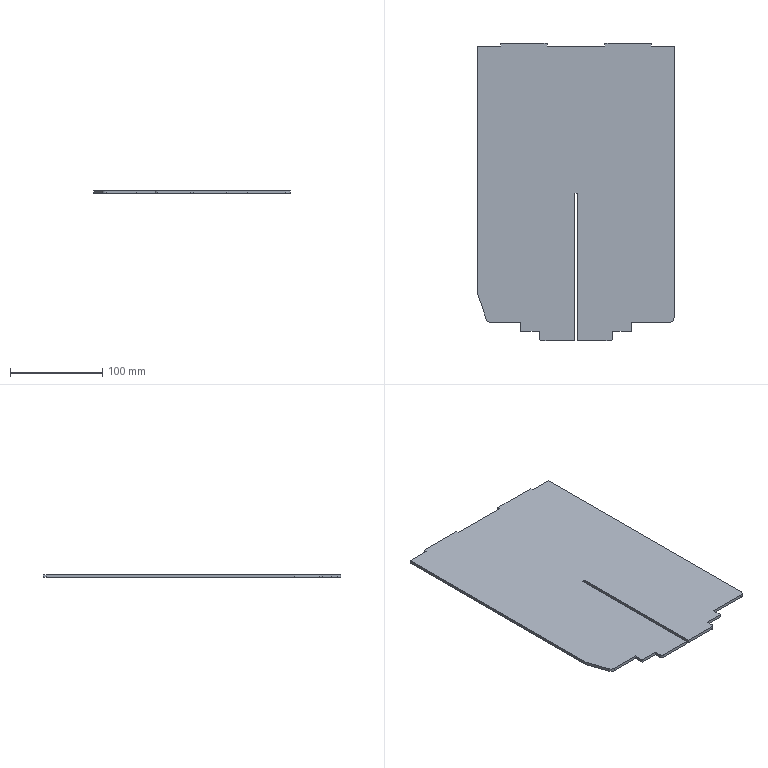Part | SolidWorks | features FlatPattern 1, SMBaseFlange 1, SheetMetal 1 | 1 solid | 31 faces | box 213 x 323 x 3.2 mm | volume 209682 mm3 | plane 27 | cylinder 4 | commonest cylinder face diameters 6 x2 10 x2
STEP:
#1=CARTESIAN_POINT('',(-107.314,104.189,0.));
#2=VERTEX_POINT('',#1);
#3=CARTESIAN_POINT('',(-132.314,104.189,0.));
#4=VERTEX_POINT('',#3);
#5=CARTESIAN_POINT('',(-107.314,104.189,0.));
#6=DIRECTION('',(-1.,0.,0.));
#7=VECTOR('',#6,1000.);
#8=LINE('',#5,#7);
#9=EDGE_CURVE('',#2,#4,#8,.T.);
#10=ORIENTED_EDGE('',*,*,#9,.T.);
#11=CARTESIAN_POINT('',(-132.314,104.189,3.2));
#12=VERTEX_POINT('',#11);
#13=CARTESIAN_POINT('',(-132.314,104.189,3.2));
#14=DIRECTION('',(0.,0.,-1.));
#15=VECTOR('',#14,1000.);
#16=LINE('',#13,#15);
#17=EDGE_CURVE('',#12,#4,#16,.T.);
#18=ORIENTED_EDGE('',*,*,#17,.F.);
#19=CARTESIAN_POINT('',(-107.314,104.189,3.2));
#20=VERTEX_POINT('',#19);
#21=CARTESIAN_POINT('',(-107.314,104.189,3.2));
#22=DIRECTION('',(-1.,0.,0.));
#23=VECTOR('',#22,1000.);
#24=LINE('',#21,#23);
#25=EDGE_CURVE('',#20,#12,#24,.T.);
#26=ORIENTED_EDGE('',*,*,#25,.F.);
#27=CARTESIAN_POINT('',(-107.314,104.189,3.2));
#28=DIRECTION('',(0.,0.,-1.));
#29=VECTOR('',#28,1000.);
#30=LINE('',#27,#29);
#31=EDGE_CURVE('',#20,#2,#30,.T.);
#32=ORIENTED_EDGE('',*,*,#31,.T.);
#33=EDGE_LOOP('',(#10,#18,#26,#32));
#34=FACE_OUTER_BOUND('',#33,.T.);
#35=CARTESIAN_POINT('',(-107.314,104.189,3.2));
#36=DIRECTION('',(0.,-1.,0.));
#37=DIRECTION('',(0.,0.,-1.));
#38=AXIS2_PLACEMENT_3D('',#35,#36,#37);
#39=PLANE('',#38);
#40=ADVANCED_FACE('',(#34),#39,.F.);
#41=CARTESIAN_POINT('',(-132.314,-165.811,0.));
#42=VERTEX_POINT('',#41);
#43=CARTESIAN_POINT('',(-132.314,-165.811,0.));
#44=DIRECTION('',(0.,-1.,0.));
#45=VECTOR('',#44,1000.);
#46=LINE('',#43,#45);
#47=EDGE_CURVE('',#4,#42,#46,.T.);
#48=ORIENTED_EDGE('',*,*,#47,.T.);
#49=CARTESIAN_POINT('',(-132.314,-165.811,3.2));
#50=VERTEX_POINT('',#49);
#51=CARTESIAN_POINT('',(-132.314,-165.811,3.2));
#52=DIRECTION('',(0.,0.,-1.));
#53=VECTOR('',#52,1000.);
#54=LINE('',#51,#53);
#55=EDGE_CURVE('',#50,#42,#54,.T.);
#56=ORIENTED_EDGE('',*,*,#55,.F.);
#57=CARTESIAN_POINT('',(-132.314,-165.811,3.2));
#58=DIRECTION('',(0.,-1.,0.));
#59=VECTOR('',#58,1000.);
#60=LINE('',#57,#59);
#61=EDGE_CURVE('',#12,#50,#60,.T.);
#62=ORIENTED_EDGE('',*,*,#61,.F.);
#63=ORIENTED_EDGE('',*,*,#17,.T.);
#64=EDGE_LOOP('',(#48,#56,#62,#63));
#65=FACE_OUTER_BOUND('',#64,.T.);
#66=CARTESIAN_POINT('',(-132.314,-165.811,3.2));
#67=DIRECTION('',(1.,0.,0.));
#68=DIRECTION('',(0.,0.,-1.));
#69=AXIS2_PLACEMENT_3D('',#66,#67,#68);
#70=PLANE('',#69);
#71=ADVANCED_FACE('',(#65),#70,.F.);
#72=CARTESIAN_POINT('',(-123.453,-192.392,0.));
#73=VERTEX_POINT('',#72);
#74=CARTESIAN_POINT('',(-123.453,-192.392,0.));
#75=DIRECTION('',(0.3162,-0.9487,0.));
#76=VECTOR('',#75,1000.);
#77=LINE('',#74,#76);
#78=EDGE_CURVE('',#42,#73,#77,.T.);
#79=ORIENTED_EDGE('',*,*,#78,.T.);
#80=CARTESIAN_POINT('',(-123.453,-192.392,3.2));
#81=VERTEX_POINT('',#80);
#82=CARTESIAN_POINT('',(-123.453,-192.392,3.2));
#83=DIRECTION('',(0.,0.,-1.));
#84=VECTOR('',#83,1000.);
#85=LINE('',#82,#84);
#86=EDGE_CURVE('',#81,#73,#85,.T.);
#87=ORIENTED_EDGE('',*,*,#86,.F.);
#88=CARTESIAN_POINT('',(-123.453,-192.392,3.2));
#89=DIRECTION('',(0.3162,-0.9487,0.));
#90=VECTOR('',#89,1000.);
#91=LINE('',#88,#90);
#92=EDGE_CURVE('',#50,#81,#91,.T.);
#93=ORIENTED_EDGE('',*,*,#92,.F.);
#94=ORIENTED_EDGE('',*,*,#55,.T.);
#95=EDGE_LOOP('',(#79,#87,#93,#94));
#96=FACE_OUTER_BOUND('',#95,.T.);
#97=CARTESIAN_POINT('',(-123.453,-192.392,3.2));
#98=DIRECTION('',(0.9487,0.3162,0.));
#99=DIRECTION('',(-0.3162,0.9487,0.));
#100=AXIS2_PLACEMENT_3D('',#97,#98,#99);
#101=PLANE('',#100);
#102=ADVANCED_FACE('',(#96),#101,.F.);
#103=CARTESIAN_POINT('',(-118.71,-195.811,0.));
#104=VERTEX_POINT('',#103);
#105=CARTESIAN_POINT('',(-118.71,-190.811,0.));
#106=DIRECTION('',(0.,0.,1.));
#107=DIRECTION('',(1.,0.,0.));
#108=AXIS2_PLACEMENT_3D('',#105,#106,#107);
#109=CIRCLE('',#108,5.);
#110=EDGE_CURVE('',#73,#104,#109,.T.);
#111=ORIENTED_EDGE('',*,*,#110,.T.);
#112=CARTESIAN_POINT('',(-118.71,-195.811,3.2));
#113=VERTEX_POINT('',#112);
#114=CARTESIAN_POINT('',(-118.71,-195.811,3.2));
#115=DIRECTION('',(0.,0.,-1.));
#116=VECTOR('',#115,1000.);
#117=LINE('',#114,#116);
#118=EDGE_CURVE('',#113,#104,#117,.T.);
#119=ORIENTED_EDGE('',*,*,#118,.F.);
#120=CARTESIAN_POINT('',(-118.71,-190.811,3.2));
#121=DIRECTION('',(0.,0.,1.));
#122=DIRECTION('',(1.,0.,0.));
#123=AXIS2_PLACEMENT_3D('',#120,#121,#122);
#124=CIRCLE('',#123,5.);
#125=EDGE_CURVE('',#81,#113,#124,.T.);
#126=ORIENTED_EDGE('',*,*,#125,.F.);
#127=ORIENTED_EDGE('',*,*,#86,.T.);
#128=EDGE_LOOP('',(#111,#119,#126,#127));
#129=FACE_OUTER_BOUND('',#128,.T.);
#130=CARTESIAN_POINT('',(-118.71,-190.811,3.2));
#131=DIRECTION('',(0.,0.,-1.));
#132=DIRECTION('',(-1.,0.,0.));
#133=AXIS2_PLACEMENT_3D('',#130,#131,#132);
#134=CYLINDRICAL_SURFACE('',#133,5.);
#135=ADVANCED_FACE('',(#129),#134,.T.);
#136=CARTESIAN_POINT('',(-85.814,-195.811,0.));
#137=VERTEX_POINT('',#136);
#138=CARTESIAN_POINT('',(-85.814,-195.811,0.));
#139=DIRECTION('',(1.,0.,0.));
#140=VECTOR('',#139,1000.);
#141=LINE('',#138,#140);
#142=EDGE_CURVE('',#104,#137,#141,.T.);
#143=ORIENTED_EDGE('',*,*,#142,.T.);
#144=CARTESIAN_POINT('',(-85.814,-195.811,3.2));
#145=VERTEX_POINT('',#144);
#146=CARTESIAN_POINT('',(-85.814,-195.811,3.2));
#147=DIRECTION('',(0.,0.,-1.));
#148=VECTOR('',#147,1000.);
#149=LINE('',#146,#148);
#150=EDGE_CURVE('',#145,#137,#149,.T.);
#151=ORIENTED_EDGE('',*,*,#150,.F.);
#152=CARTESIAN_POINT('',(-85.814,-195.811,3.2));
#153=DIRECTION('',(1.,0.,0.));
#154=VECTOR('',#153,1000.);
#155=LINE('',#152,#154);
#156=EDGE_CURVE('',#113,#145,#155,.T.);
#157=ORIENTED_EDGE('',*,*,#156,.F.);
#158=ORIENTED_EDGE('',*,*,#118,.T.);
#159=EDGE_LOOP('',(#143,#151,#157,#158));
#160=FACE_OUTER_BOUND('',#159,.T.);
#161=CARTESIAN_POINT('',(-85.814,-195.811,3.2));
#162=DIRECTION('',(0.,1.,0.));
#163=DIRECTION('',(-1.,0.,0.));
#164=AXIS2_PLACEMENT_3D('',#161,#162,#163);
#165=PLANE('',#164);
#166=ADVANCED_FACE('',(#160),#165,.F.);
#167=CARTESIAN_POINT('',(-85.814,-205.811,0.));
#168=VERTEX_POINT('',#167);
#169=CARTESIAN_POINT('',(-85.814,-205.811,0.));
#170=DIRECTION('',(0.,-1.,0.));
#171=VECTOR('',#170,1000.);
#172=LINE('',#169,#171);
#173=EDGE_CURVE('',#137,#168,#172,.T.);
#174=ORIENTED_EDGE('',*,*,#173,.T.);
#175=CARTESIAN_POINT('',(-85.814,-205.811,3.2));
#176=VERTEX_POINT('',#175);
#177=CARTESIAN_POINT('',(-85.814,-205.811,3.2));
#178=DIRECTION('',(0.,0.,-1.));
#179=VECTOR('',#178,1000.);
#180=LINE('',#177,#179);
#181=EDGE_CURVE('',#176,#168,#180,.T.);
#182=ORIENTED_EDGE('',*,*,#181,.F.);
#183=CARTESIAN_POINT('',(-85.814,-205.811,3.2));
#184=DIRECTION('',(0.,-1.,0.));
#185=VECTOR('',#184,1000.);
#186=LINE('',#183,#185);
#187=EDGE_CURVE('',#145,#176,#186,.T.);
#188=ORIENTED_EDGE('',*,*,#187,.F.);
#189=ORIENTED_EDGE('',*,*,#150,.T.);
#190=EDGE_LOOP('',(#174,#182,#188,#189));
#191=FACE_OUTER_BOUND('',#190,.T.);
#192=CARTESIAN_POINT('',(-85.814,-205.811,3.2));
#193=DIRECTION('',(1.,0.,0.));
#194=DIRECTION('',(0.,1.,0.));
#195=AXIS2_PLACEMENT_3D('',#192,#193,#194);
#196=PLANE('',#195);
#197=ADVANCED_FACE('',(#191),#196,.F.);
#198=CARTESIAN_POINT('',(-65.814,-205.811,0.));
#199=VERTEX_POINT('',#198);
#200=CARTESIAN_POINT('',(-65.814,-205.811,0.));
#201=DIRECTION('',(1.,0.,0.));
#202=VECTOR('',#201,1000.);
#203=LINE('',#200,#202);
#204=EDGE_CURVE('',#168,#199,#203,.T.);
#205=ORIENTED_EDGE('',*,*,#204,.T.);
#206=CARTESIAN_POINT('',(-65.814,-205.811,3.2));
#207=VERTEX_POINT('',#206);
#208=CARTESIAN_POINT('',(-65.814,-205.811,3.2));
#209=DIRECTION('',(0.,0.,-1.));
#210=VECTOR('',#209,1000.);
#211=LINE('',#208,#210);
#212=EDGE_CURVE('',#207,#199,#211,.T.);
#213=ORIENTED_EDGE('',*,*,#212,.F.);
#214=CARTESIAN_POINT('',(-65.814,-205.811,3.2));
#215=DIRECTION('',(1.,0.,0.));
#216=VECTOR('',#215,1000.);
#217=LINE('',#214,#216);
#218=EDGE_CURVE('',#176,#207,#217,.T.);
#219=ORIENTED_EDGE('',*,*,#218,.F.);
#220=ORIENTED_EDGE('',*,*,#181,.T.);
#221=EDGE_LOOP('',(#205,#213,#219,#220));
#222=FACE_OUTER_BOUND('',#221,.T.);
#223=CARTESIAN_POINT('',(-65.814,-205.811,3.2));
#224=DIRECTION('',(0.,1.,0.));
#225=DIRECTION('',(-1.,0.,0.));
#226=AXIS2_PLACEMENT_3D('',#223,#224,#225);
#227=PLANE('',#226);
#228=ADVANCED_FACE('',(#222),#227,.F.);
#229=CARTESIAN_POINT('',(-65.814,-212.811,0.));
#230=VERTEX_POINT('',#229);
#231=CARTESIAN_POINT('',(-65.814,-212.811,0.));
#232=DIRECTION('',(0.,-1.,0.));
#233=VECTOR('',#232,1000.);
#234=LINE('',#231,#233);
#235=EDGE_CURVE('',#199,#230,#234,.T.);
#236=ORIENTED_EDGE('',*,*,#235,.T.);
#237=CARTESIAN_POINT('',(-65.814,-212.811,3.2));
#238=VERTEX_POINT('',#237);
#239=CARTESIAN_POINT('',(-65.814,-212.811,3.2));
#240=DIRECTION('',(0.,0.,-1.));
#241=VECTOR('',#240,1000.);
#242=LINE('',#239,#241);
#243=EDGE_CURVE('',#238,#230,#242,.T.);
#244=ORIENTED_EDGE('',*,*,#243,.F.);
#245=CARTESIAN_POINT('',(-65.814,-212.811,3.2));
#246=DIRECTION('',(0.,-1.,0.));
#247=VECTOR('',#246,1000.);
#248=LINE('',#245,#247);
#249=EDGE_CURVE('',#207,#238,#248,.T.);
#250=ORIENTED_EDGE('',*,*,#249,.F.);
#251=ORIENTED_EDGE('',*,*,#212,.T.);
#252=EDGE_LOOP('',(#236,#244,#250,#251));
#253=FACE_OUTER_BOUND('',#252,.T.);
#254=CARTESIAN_POINT('',(-65.814,-212.811,3.2));
#255=DIRECTION('',(1.,0.,0.));
#256=DIRECTION('',(0.,0.,-1.));
#257=AXIS2_PLACEMENT_3D('',#254,#255,#256);
#258=PLANE('',#257);
#259=ADVANCED_FACE('',(#253),#258,.F.);
#260=CARTESIAN_POINT('',(-62.814,-215.811,0.));
#261=VERTEX_POINT('',#260);
#262=CARTESIAN_POINT('',(-62.814,-212.811,0.));
#263=DIRECTION('',(0.,0.,1.));
#264=DIRECTION('',(-1.,0.,0.));
#265=AXIS2_PLACEMENT_3D('',#262,#263,#264);
#266=CIRCLE('',#265,3.);
#267=EDGE_CURVE('',#230,#261,#266,.T.);
#268=ORIENTED_EDGE('',*,*,#267,.T.);
#269=CARTESIAN_POINT('',(-62.814,-215.811,3.2));
#270=VERTEX_POINT('',#269);
#271=CARTESIAN_POINT('',(-62.814,-215.811,3.2));
#272=DIRECTION('',(0.,0.,-1.));
#273=VECTOR('',#272,1000.);
#274=LINE('',#271,#273);
#275=EDGE_CURVE('',#270,#261,#274,.T.);
#276=ORIENTED_EDGE('',*,*,#275,.F.);
#277=CARTESIAN_POINT('',(-62.814,-212.811,3.2));
#278=DIRECTION('',(0.,0.,1.));
#279=DIRECTION('',(-1.,0.,0.));
#280=AXIS2_PLACEMENT_3D('',#277,#278,#279);
#281=CIRCLE('',#280,3.);
#282=EDGE_CURVE('',#238,#270,#281,.T.);
#283=ORIENTED_EDGE('',*,*,#282,.F.);
#284=ORIENTED_EDGE('',*,*,#243,.T.);
#285=EDGE_LOOP('',(#268,#276,#283,#284));
#286=FACE_OUTER_BOUND('',#285,.T.);
#287=CARTESIAN_POINT('',(-62.814,-212.811,3.2));
#288=DIRECTION('',(0.,0.,-1.));
#289=DIRECTION('',(-1.,0.,0.));
#290=AXIS2_PLACEMENT_3D('',#287,#288,#289);
#291=CYLINDRICAL_SURFACE('',#290,3.);
#292=ADVANCED_FACE('',(#286),#291,.T.);
#293=CARTESIAN_POINT('',(-27.414,-215.811,0.));
#294=VERTEX_POINT('',#293);
#295=CARTESIAN_POINT('',(-27.414,-215.811,0.));
#296=DIRECTION('',(1.,0.,0.));
#297=VECTOR('',#296,1000.);
#298=LINE('',#295,#297);
#299=EDGE_CURVE('',#261,#294,#298,.T.);
#300=ORIENTED_EDGE('',*,*,#299,.T.);
#301=CARTESIAN_POINT('',(-27.414,-215.811,3.2));
#302=VERTEX_POINT('',#301);
#303=CARTESIAN_POINT('',(-27.414,-215.811,3.2));
#304=DIRECTION('',(0.,0.,-1.));
#305=VECTOR('',#304,1000.);
#306=LINE('',#303,#305);
#307=EDGE_CURVE('',#302,#294,#306,.T.);
#308=ORIENTED_EDGE('',*,*,#307,.F.);
#309=CARTESIAN_POINT('',(-27.414,-215.811,3.2));
#310=DIRECTION('',(1.,0.,0.));
#311=VECTOR('',#310,1000.);
#312=LINE('',#309,#311);
#313=EDGE_CURVE('',#270,#302,#312,.T.);
#314=ORIENTED_EDGE('',*,*,#313,.F.);
#315=ORIENTED_EDGE('',*,*,#275,.T.);
#316=EDGE_LOOP('',(#300,#308,#314,#315));
#317=FACE_OUTER_BOUND('',#316,.T.);
#318=CARTESIAN_POINT('',(-27.414,-215.811,3.2));
#319=DIRECTION('',(0.,1.,0.));
#320=DIRECTION('',(0.,0.,1.));
#321=AXIS2_PLACEMENT_3D('',#318,#319,#320);
#322=PLANE('',#321);
#323=ADVANCED_FACE('',(#317),#322,.F.);
#324=CARTESIAN_POINT('',(-27.414,-55.611,0.));
#325=VERTEX_POINT('',#324);
#326=CARTESIAN_POINT('',(-27.414,-55.611,0.));
#327=DIRECTION('',(0.,1.,0.));
#328=VECTOR('',#327,1000.);
#329=LINE('',#326,#328);
#330=EDGE_CURVE('',#294,#325,#329,.T.);
#331=ORIENTED_EDGE('',*,*,#330,.T.);
#332=CARTESIAN_POINT('',(-27.414,-55.611,3.2));
#333=VERTEX_POINT('',#332);
#334=CARTESIAN_POINT('',(-27.414,-55.611,3.2));
#335=DIRECTION('',(0.,0.,-1.));
#336=VECTOR('',#335,1000.);
#337=LINE('',#334,#336);
#338=EDGE_CURVE('',#333,#325,#337,.T.);
#339=ORIENTED_EDGE('',*,*,#338,.F.);
#340=CARTESIAN_POINT('',(-27.414,-55.611,3.2));
#341=DIRECTION('',(0.,1.,0.));
#342=VECTOR('',#341,1000.);
#343=LINE('',#340,#342);
#344=EDGE_CURVE('',#302,#333,#343,.T.);
#345=ORIENTED_EDGE('',*,*,#344,.F.);
#346=ORIENTED_EDGE('',*,*,#307,.T.);
#347=EDGE_LOOP('',(#331,#339,#345,#346));
#348=FACE_OUTER_BOUND('',#347,.T.);
#349=CARTESIAN_POINT('',(-27.414,-55.611,3.2));
#350=DIRECTION('',(-1.,0.,0.));
#351=DIRECTION('',(0.,0.,1.));
#352=AXIS2_PLACEMENT_3D('',#349,#350,#351);
#353=PLANE('',#352);
#354=ADVANCED_FACE('',(#348),#353,.F.);
#355=CARTESIAN_POINT('',(-24.214,-55.611,0.));
#356=VERTEX_POINT('',#355);
#357=CARTESIAN_POINT('',(-24.214,-55.611,0.));
#358=DIRECTION('',(1.,0.,0.));
#359=VECTOR('',#358,1000.);
#360=LINE('',#357,#359);
#361=EDGE_CURVE('',#325,#356,#360,.T.);
#362=ORIENTED_EDGE('',*,*,#361,.T.);
#363=CARTESIAN_POINT('',(-24.214,-55.611,3.2));
#364=VERTEX_POINT('',#363);
#365=CARTESIAN_POINT('',(-24.214,-55.611,3.2));
#366=DIRECTION('',(0.,0.,-1.));
#367=VECTOR('',#366,1000.);
#368=LINE('',#365,#367);
#369=EDGE_CURVE('',#364,#356,#368,.T.);
#370=ORIENTED_EDGE('',*,*,#369,.F.);
#371=CARTESIAN_POINT('',(-24.214,-55.611,3.2));
#372=DIRECTION('',(1.,0.,0.));
#373=VECTOR('',#372,1000.);
#374=LINE('',#371,#373);
#375=EDGE_CURVE('',#333,#364,#374,.T.);
#376=ORIENTED_EDGE('',*,*,#375,.F.);
#377=ORIENTED_EDGE('',*,*,#338,.T.);
#378=EDGE_LOOP('',(#362,#370,#376,#377));
#379=FACE_OUTER_BOUND('',#378,.T.);
#380=CARTESIAN_POINT('',(-24.214,-55.611,3.2));
#381=DIRECTION('',(0.,1.,0.));
#382=DIRECTION('',(-1.,0.,0.));
#383=AXIS2_PLACEMENT_3D('',#380,#381,#382);
#384=PLANE('',#383);
#385=ADVANCED_FACE('',(#379),#384,.F.);
#386=CARTESIAN_POINT('',(-24.214,-215.811,0.));
#387=VERTEX_POINT('',#386);
#388=CARTESIAN_POINT('',(-24.214,-215.811,0.));
#389=DIRECTION('',(0.,-1.,0.));
#390=VECTOR('',#389,1000.);
#391=LINE('',#388,#390);
#392=EDGE_CURVE('',#356,#387,#391,.T.);
#393=ORIENTED_EDGE('',*,*,#392,.T.);
#394=CARTESIAN_POINT('',(-24.214,-215.811,3.2));
#395=VERTEX_POINT('',#394);
#396=CARTESIAN_POINT('',(-24.214,-215.811,3.2));
#397=DIRECTION('',(0.,0.,-1.));
#398=VECTOR('',#397,1000.);
#399=LINE('',#396,#398);
#400=EDGE_CURVE('',#395,#387,#399,.T.);
#401=ORIENTED_EDGE('',*,*,#400,.F.);
#402=CARTESIAN_POINT('',(-24.214,-215.811,3.2));
#403=DIRECTION('',(0.,-1.,0.));
#404=VECTOR('',#403,1000.);
#405=LINE('',#402,#404);
#406=EDGE_CURVE('',#364,#395,#405,.T.);
#407=ORIENTED_EDGE('',*,*,#406,.F.);
#408=ORIENTED_EDGE('',*,*,#369,.T.);
#409=EDGE_LOOP('',(#393,#401,#407,#408));
#410=FACE_OUTER_BOUND('',#409,.T.);
#411=CARTESIAN_POINT('',(-24.214,-215.811,3.2));
#412=DIRECTION('',(1.,0.,0.));
#413=DIRECTION('',(0.,1.,0.));
#414=AXIS2_PLACEMENT_3D('',#411,#412,#413);
#415=PLANE('',#414);
#416=ADVANCED_FACE('',(#410),#415,.F.);
#417=CARTESIAN_POINT('',(11.186,-215.811,0.));
#418=VERTEX_POINT('',#417);
#419=CARTESIAN_POINT('',(11.186,-215.811,0.));
#420=DIRECTION('',(1.,0.,0.));
#421=VECTOR('',#420,1000.);
#422=LINE('',#419,#421);
#423=EDGE_CURVE('',#387,#418,#422,.T.);
#424=ORIENTED_EDGE('',*,*,#423,.T.);
#425=CARTESIAN_POINT('',(11.186,-215.811,3.2));
#426=VERTEX_POINT('',#425);
#427=CARTESIAN_POINT('',(11.186,-215.811,3.2));
#428=DIRECTION('',(0.,0.,-1.));
#429=VECTOR('',#428,1000.);
#430=LINE('',#427,#429);
#431=EDGE_CURVE('',#426,#418,#430,.T.);
#432=ORIENTED_EDGE('',*,*,#431,.F.);
#433=CARTESIAN_POINT('',(11.186,-215.811,3.2));
#434=DIRECTION('',(1.,0.,0.));
#435=VECTOR('',#434,1000.);
#436=LINE('',#433,#435);
#437=EDGE_CURVE('',#395,#426,#436,.T.);
#438=ORIENTED_EDGE('',*,*,#437,.F.);
#439=ORIENTED_EDGE('',*,*,#400,.T.);
#440=EDGE_LOOP('',(#424,#432,#438,#439));
#441=FACE_OUTER_BOUND('',#440,.T.);
#442=CARTESIAN_POINT('',(11.186,-215.811,3.2));
#443=DIRECTION('',(0.,1.,0.));
#444=DIRECTION('',(-1.,0.,0.));
#445=AXIS2_PLACEMENT_3D('',#442,#443,#444);
#446=PLANE('',#445);
#447=ADVANCED_FACE('',(#441),#446,.F.);
#448=CARTESIAN_POINT('',(14.186,-212.811,0.));
#449=VERTEX_POINT('',#448);
#450=CARTESIAN_POINT('',(11.186,-212.811,0.));
#451=DIRECTION('',(0.,0.,1.));
#452=DIRECTION('',(-1.,0.,0.));
#453=AXIS2_PLACEMENT_3D('',#450,#451,#452);
#454=CIRCLE('',#453,3.);
#455=EDGE_CURVE('',#418,#449,#454,.T.);
#456=ORIENTED_EDGE('',*,*,#455,.T.);
#457=CARTESIAN_POINT('',(14.186,-212.811,3.2));
#458=VERTEX_POINT('',#457);
#459=CARTESIAN_POINT('',(14.186,-212.811,3.2));
#460=DIRECTION('',(0.,0.,-1.));
#461=VECTOR('',#460,1000.);
#462=LINE('',#459,#461);
#463=EDGE_CURVE('',#458,#449,#462,.T.);
#464=ORIENTED_EDGE('',*,*,#463,.F.);
#465=CARTESIAN_POINT('',(11.186,-212.811,3.2));
#466=DIRECTION('',(0.,0.,1.));
#467=DIRECTION('',(-1.,0.,0.));
#468=AXIS2_PLACEMENT_3D('',#465,#466,#467);
#469=CIRCLE('',#468,3.);
#470=EDGE_CURVE('',#426,#458,#469,.T.);
#471=ORIENTED_EDGE('',*,*,#470,.F.);
#472=ORIENTED_EDGE('',*,*,#431,.T.);
#473=EDGE_LOOP('',(#456,#464,#471,#472));
#474=FACE_OUTER_BOUND('',#473,.T.);
#475=CARTESIAN_POINT('',(11.186,-212.811,3.2));
#476=DIRECTION('',(0.,0.,-1.));
#477=DIRECTION('',(-1.,0.,0.));
#478=AXIS2_PLACEMENT_3D('',#475,#476,#477);
#479=CYLINDRICAL_SURFACE('',#478,3.);
#480=ADVANCED_FACE('',(#474),#479,.T.);
#481=CARTESIAN_POINT('',(14.186,-205.811,0.));
#482=VERTEX_POINT('',#481);
#483=CARTESIAN_POINT('',(14.186,-205.811,0.));
#484=DIRECTION('',(0.,1.,0.));
#485=VECTOR('',#484,1000.);
#486=LINE('',#483,#485);
#487=EDGE_CURVE('',#449,#482,#486,.T.);
#488=ORIENTED_EDGE('',*,*,#487,.T.);
#489=CARTESIAN_POINT('',(14.186,-205.811,3.2));
#490=VERTEX_POINT('',#489);
#491=CARTESIAN_POINT('',(14.186,-205.811,3.2));
#492=DIRECTION('',(0.,0.,-1.));
#493=VECTOR('',#492,1000.);
#494=LINE('',#491,#493);
#495=EDGE_CURVE('',#490,#482,#494,.T.);
#496=ORIENTED_EDGE('',*,*,#495,.F.);
#497=CARTESIAN_POINT('',(14.186,-205.811,3.2));
#498=DIRECTION('',(0.,1.,0.));
#499=VECTOR('',#498,1000.);
#500=LINE('',#497,#499);
#501=EDGE_CURVE('',#458,#490,#500,.T.);
#502=ORIENTED_EDGE('',*,*,#501,.F.);
#503=ORIENTED_EDGE('',*,*,#463,.T.);
#504=EDGE_LOOP('',(#488,#496,#502,#503));
#505=FACE_OUTER_BOUND('',#504,.T.);
#506=CARTESIAN_POINT('',(14.186,-205.811,3.2));
#507=DIRECTION('',(-1.,0.,0.));
#508=DIRECTION('',(0.,-1.,0.));
#509=AXIS2_PLACEMENT_3D('',#506,#507,#508);
#510=PLANE('',#509);
#511=ADVANCED_FACE('',(#505),#510,.F.);
#512=CARTESIAN_POINT('',(34.186,-205.811,0.));
#513=VERTEX_POINT('',#512);
#514=CARTESIAN_POINT('',(34.186,-205.811,0.));
#515=DIRECTION('',(1.,0.,0.));
#516=VECTOR('',#515,1000.);
#517=LINE('',#514,#516);
#518=EDGE_CURVE('',#482,#513,#517,.T.);
#519=ORIENTED_EDGE('',*,*,#518,.T.);
#520=CARTESIAN_POINT('',(34.186,-205.811,3.2));
#521=VERTEX_POINT('',#520);
#522=CARTESIAN_POINT('',(34.186,-205.811,3.2));
#523=DIRECTION('',(0.,0.,-1.));
#524=VECTOR('',#523,1000.);
#525=LINE('',#522,#524);
#526=EDGE_CURVE('',#521,#513,#525,.T.);
#527=ORIENTED_EDGE('',*,*,#526,.F.);
#528=CARTESIAN_POINT('',(34.186,-205.811,3.2));
#529=DIRECTION('',(1.,0.,0.));
#530=VECTOR('',#529,1000.);
#531=LINE('',#528,#530);
#532=EDGE_CURVE('',#490,#521,#531,.T.);
#533=ORIENTED_EDGE('',*,*,#532,.F.);
#534=ORIENTED_EDGE('',*,*,#495,.T.);
#535=EDGE_LOOP('',(#519,#527,#533,#534));
#536=FACE_OUTER_BOUND('',#535,.T.);
#537=CARTESIAN_POINT('',(34.186,-205.811,3.2));
#538=DIRECTION('',(0.,1.,0.));
#539=DIRECTION('',(-1.,0.,0.));
#540=AXIS2_PLACEMENT_3D('',#537,#538,#539);
#541=PLANE('',#540);
#542=ADVANCED_FACE('',(#536),#541,.F.);
#543=CARTESIAN_POINT('',(34.186,-195.811,0.));
#544=VERTEX_POINT('',#543);
#545=CARTESIAN_POINT('',(34.186,-195.811,0.));
#546=DIRECTION('',(0.,1.,0.));
#547=VECTOR('',#546,1000.);
#548=LINE('',#545,#547);
#549=EDGE_CURVE('',#513,#544,#548,.T.);
#550=ORIENTED_EDGE('',*,*,#549,.T.);
#551=CARTESIAN_POINT('',(34.186,-195.811,3.2));
#552=VERTEX_POINT('',#551);
#553=CARTESIAN_POINT('',(34.186,-195.811,3.2));
#554=DIRECTION('',(0.,0.,-1.));
#555=VECTOR('',#554,1000.);
#556=LINE('',#553,#555);
#557=EDGE_CURVE('',#552,#544,#556,.T.);
#558=ORIENTED_EDGE('',*,*,#557,.F.);
#559=CARTESIAN_POINT('',(34.186,-195.811,3.2));
#560=DIRECTION('',(0.,1.,0.));
#561=VECTOR('',#560,1000.);
#562=LINE('',#559,#561);
#563=EDGE_CURVE('',#521,#552,#562,.T.);
#564=ORIENTED_EDGE('',*,*,#563,.F.);
#565=ORIENTED_EDGE('',*,*,#526,.T.);
#566=EDGE_LOOP('',(#550,#558,#564,#565));
#567=FACE_OUTER_BOUND('',#566,.T.);
#568=CARTESIAN_POINT('',(34.186,-195.811,3.2));
#569=DIRECTION('',(-1.,0.,0.));
#570=DIRECTION('',(0.,-1.,0.));
#571=AXIS2_PLACEMENT_3D('',#568,#569,#570);
#572=PLANE('',#571);
#573=ADVANCED_FACE('',(#567),#572,.F.);
#574=CARTESIAN_POINT('',(75.686,-195.811,0.));
#575=VERTEX_POINT('',#574);
#576=CARTESIAN_POINT('',(75.686,-195.811,0.));
#577=DIRECTION('',(1.,0.,0.));
#578=VECTOR('',#577,1000.);
#579=LINE('',#576,#578);
#580=EDGE_CURVE('',#544,#575,#579,.T.);
#581=ORIENTED_EDGE('',*,*,#580,.T.);
#582=CARTESIAN_POINT('',(75.686,-195.811,3.2));
#583=VERTEX_POINT('',#582);
#584=CARTESIAN_POINT('',(75.686,-195.811,3.2));
#585=DIRECTION('',(0.,0.,-1.));
#586=VECTOR('',#585,1000.);
#587=LINE('',#584,#586);
#588=EDGE_CURVE('',#583,#575,#587,.T.);
#589=ORIENTED_EDGE('',*,*,#588,.F.);
#590=CARTESIAN_POINT('',(75.686,-195.811,3.2));
#591=DIRECTION('',(1.,0.,0.));
#592=VECTOR('',#591,1000.);
#593=LINE('',#590,#592);
#594=EDGE_CURVE('',#552,#583,#593,.T.);
#595=ORIENTED_EDGE('',*,*,#594,.F.);
#596=ORIENTED_EDGE('',*,*,#557,.T.);
#597=EDGE_LOOP('',(#581,#589,#595,#596));
#598=FACE_OUTER_BOUND('',#597,.T.);
#599=CARTESIAN_POINT('',(75.686,-195.811,3.2));
#600=DIRECTION('',(0.,1.,0.));
#601=DIRECTION('',(-1.,0.,0.));
#602=AXIS2_PLACEMENT_3D('',#599,#600,#601);
#603=PLANE('',#602);
#604=ADVANCED_FACE('',(#598),#603,.F.);
#605=CARTESIAN_POINT('',(80.686,-190.811,0.));
#606=VERTEX_POINT('',#605);
#607=CARTESIAN_POINT('',(75.686,-190.811,0.));
#608=DIRECTION('',(0.,0.,1.));
#609=DIRECTION('',(1.,0.,0.));
#610=AXIS2_PLACEMENT_3D('',#607,#608,#609);
#611=CIRCLE('',#610,5.);
#612=EDGE_CURVE('',#575,#606,#611,.T.);
#613=ORIENTED_EDGE('',*,*,#612,.T.);
#614=CARTESIAN_POINT('',(80.686,-190.811,3.2));
#615=VERTEX_POINT('',#614);
#616=CARTESIAN_POINT('',(80.686,-190.811,3.2));
#617=DIRECTION('',(0.,0.,-1.));
#618=VECTOR('',#617,1000.);
#619=LINE('',#616,#618);
#620=EDGE_CURVE('',#615,#606,#619,.T.);
#621=ORIENTED_EDGE('',*,*,#620,.F.);
#622=CARTESIAN_POINT('',(75.686,-190.811,3.2));
#623=DIRECTION('',(0.,0.,1.));
#624=DIRECTION('',(1.,0.,0.));
#625=AXIS2_PLACEMENT_3D('',#622,#623,#624);
#626=CIRCLE('',#625,5.);
#627=EDGE_CURVE('',#583,#615,#626,.T.);
#628=ORIENTED_EDGE('',*,*,#627,.F.);
#629=ORIENTED_EDGE('',*,*,#588,.T.);
#630=EDGE_LOOP('',(#613,#621,#628,#629));
#631=FACE_OUTER_BOUND('',#630,.T.);
#632=CARTESIAN_POINT('',(75.686,-190.811,3.2));
#633=DIRECTION('',(0.,0.,-1.));
#634=DIRECTION('',(-1.,0.,0.));
#635=AXIS2_PLACEMENT_3D('',#632,#633,#634);
#636=CYLINDRICAL_SURFACE('',#635,5.);
#637=ADVANCED_FACE('',(#631),#636,.T.);
#638=CARTESIAN_POINT('',(80.686,104.189,0.));
#639=VERTEX_POINT('',#638);
#640=CARTESIAN_POINT('',(80.686,-190.811,0.));
#641=DIRECTION('',(0.,1.,0.));
#642=VECTOR('',#641,1000.);
#643=LINE('',#640,#642);
#644=EDGE_CURVE('',#606,#639,#643,.T.);
#645=ORIENTED_EDGE('',*,*,#644,.T.);
#646=CARTESIAN_POINT('',(80.686,104.189,3.2));
#647=VERTEX_POINT('',#646);
#648=CARTESIAN_POINT('',(80.686,104.189,3.2));
#649=DIRECTION('',(0.,0.,-1.));
#650=VECTOR('',#649,1000.);
#651=LINE('',#648,#650);
#652=EDGE_CURVE('',#647,#639,#651,.T.);
#653=ORIENTED_EDGE('',*,*,#652,.F.);
#654=CARTESIAN_POINT('',(80.686,-190.811,3.2));
#655=DIRECTION('',(0.,1.,0.));
#656=VECTOR('',#655,1000.);
#657=LINE('',#654,#656);
#658=EDGE_CURVE('',#615,#647,#657,.T.);
#659=ORIENTED_EDGE('',*,*,#658,.F.);
#660=ORIENTED_EDGE('',*,*,#620,.T.);
#661=EDGE_LOOP('',(#645,#653,#659,#660));
#662=FACE_OUTER_BOUND('',#661,.T.);
#663=CARTESIAN_POINT('',(80.686,-190.811,3.2));
#664=DIRECTION('',(-1.,0.,0.));
#665=DIRECTION('',(0.,0.,1.));
#666=AXIS2_PLACEMENT_3D('',#663,#664,#665);
#667=PLANE('',#666);
#668=ADVANCED_FACE('',(#662),#667,.F.);
#669=CARTESIAN_POINT('',(55.686,104.189,0.));
#670=VERTEX_POINT('',#669);
#671=CARTESIAN_POINT('',(80.686,104.189,0.));
#672=DIRECTION('',(-1.,0.,0.));
#673=VECTOR('',#672,1000.);
#674=LINE('',#671,#673);
#675=EDGE_CURVE('',#639,#670,#674,.T.);
#676=ORIENTED_EDGE('',*,*,#675,.T.);
#677=CARTESIAN_POINT('',(55.686,104.189,3.2));
#678=VERTEX_POINT('',#677);
#679=CARTESIAN_POINT('',(55.686,104.189,3.2));
#680=DIRECTION('',(0.,0.,-1.));
#681=VECTOR('',#680,1000.);
#682=LINE('',#679,#681);
#683=EDGE_CURVE('',#678,#670,#682,.T.);
#684=ORIENTED_EDGE('',*,*,#683,.F.);
#685=CARTESIAN_POINT('',(80.686,104.189,3.2));
#686=DIRECTION('',(-1.,0.,0.));
#687=VECTOR('',#686,1000.);
#688=LINE('',#685,#687);
#689=EDGE_CURVE('',#647,#678,#688,.T.);
#690=ORIENTED_EDGE('',*,*,#689,.F.);
#691=ORIENTED_EDGE('',*,*,#652,.T.);
#692=EDGE_LOOP('',(#676,#684,#690,#691));
#693=FACE_OUTER_BOUND('',#692,.T.);
#694=CARTESIAN_POINT('',(80.686,104.189,3.2));
#695=DIRECTION('',(0.,-1.,0.));
#696=DIRECTION('',(1.,0.,0.));
#697=AXIS2_PLACEMENT_3D('',#694,#695,#696);
#698=PLANE('',#697);
#699=ADVANCED_FACE('',(#693),#698,.F.);
#700=CARTESIAN_POINT('',(55.686,107.189,0.));
#701=VERTEX_POINT('',#700);
#702=CARTESIAN_POINT('',(55.686,104.189,0.));
#703=DIRECTION('',(0.,1.,0.));
#704=VECTOR('',#703,1000.);
#705=LINE('',#702,#704);
#706=EDGE_CURVE('',#670,#701,#705,.T.);
#707=ORIENTED_EDGE('',*,*,#706,.T.);
#708=CARTESIAN_POINT('',(55.686,107.189,3.2));
#709=VERTEX_POINT('',#708);
#710=CARTESIAN_POINT('',(55.686,107.189,3.2));
#711=DIRECTION('',(0.,0.,-1.));
#712=VECTOR('',#711,1000.);
#713=LINE('',#710,#712);
#714=EDGE_CURVE('',#709,#701,#713,.T.);
#715=ORIENTED_EDGE('',*,*,#714,.F.);
#716=CARTESIAN_POINT('',(55.686,104.189,3.2));
#717=DIRECTION('',(0.,1.,0.));
#718=VECTOR('',#717,1000.);
#719=LINE('',#716,#718);
#720=EDGE_CURVE('',#678,#709,#719,.T.);
#721=ORIENTED_EDGE('',*,*,#720,.F.);
#722=ORIENTED_EDGE('',*,*,#683,.T.);
#723=EDGE_LOOP('',(#707,#715,#721,#722));
#724=FACE_OUTER_BOUND('',#723,.T.);
#725=CARTESIAN_POINT('',(55.686,104.189,3.2));
#726=DIRECTION('',(-1.,0.,0.));
#727=DIRECTION('',(0.,0.,1.));
#728=AXIS2_PLACEMENT_3D('',#725,#726,#727);
#729=PLANE('',#728);
#730=ADVANCED_FACE('',(#724),#729,.F.);
#731=CARTESIAN_POINT('',(5.686,107.189,0.));
#732=VERTEX_POINT('',#731);
#733=CARTESIAN_POINT('',(55.686,107.189,0.));
#734=DIRECTION('',(-1.,0.,0.));
#735=VECTOR('',#734,1000.);
#736=LINE('',#733,#735);
#737=EDGE_CURVE('',#701,#732,#736,.T.);
#738=ORIENTED_EDGE('',*,*,#737,.T.);
#739=CARTESIAN_POINT('',(5.686,107.189,3.2));
#740=VERTEX_POINT('',#739);
#741=CARTESIAN_POINT('',(5.686,107.189,3.2));
#742=DIRECTION('',(0.,0.,-1.));
#743=VECTOR('',#742,1000.);
#744=LINE('',#741,#743);
#745=EDGE_CURVE('',#740,#732,#744,.T.);
#746=ORIENTED_EDGE('',*,*,#745,.F.);
#747=CARTESIAN_POINT('',(55.686,107.189,3.2));
#748=DIRECTION('',(-1.,0.,0.));
#749=VECTOR('',#748,1000.);
#750=LINE('',#747,#749);
#751=EDGE_CURVE('',#709,#740,#750,.T.);
#752=ORIENTED_EDGE('',*,*,#751,.F.);
#753=ORIENTED_EDGE('',*,*,#714,.T.);
#754=EDGE_LOOP('',(#738,#746,#752,#753));
#755=FACE_OUTER_BOUND('',#754,.T.);
#756=CARTESIAN_POINT('',(55.686,107.189,3.2));
#757=DIRECTION('',(0.,-1.,0.));
#758=DIRECTION('',(0.,0.,-1.));
#759=AXIS2_PLACEMENT_3D('',#756,#757,#758);
#760=PLANE('',#759);
#761=ADVANCED_FACE('',(#755),#760,.F.);
#762=CARTESIAN_POINT('',(5.686,104.189,0.));
#763=VERTEX_POINT('',#762);
#764=CARTESIAN_POINT('',(5.686,107.189,0.));
#765=DIRECTION('',(0.,-1.,0.));
#766=VECTOR('',#765,1000.);
#767=LINE('',#764,#766);
#768=EDGE_CURVE('',#732,#763,#767,.T.);
#769=ORIENTED_EDGE('',*,*,#768,.T.);
#770=CARTESIAN_POINT('',(5.686,104.189,3.2));
#771=VERTEX_POINT('',#770);
#772=CARTESIAN_POINT('',(5.686,104.189,3.2));
#773=DIRECTION('',(0.,0.,-1.));
#774=VECTOR('',#773,1000.);
#775=LINE('',#772,#774);
#776=EDGE_CURVE('',#771,#763,#775,.T.);
#777=ORIENTED_EDGE('',*,*,#776,.F.);
#778=CARTESIAN_POINT('',(5.686,107.189,3.2));
#779=DIRECTION('',(0.,-1.,0.));
#780=VECTOR('',#779,1000.);
#781=LINE('',#778,#780);
#782=EDGE_CURVE('',#740,#771,#781,.T.);
#783=ORIENTED_EDGE('',*,*,#782,.F.);
#784=ORIENTED_EDGE('',*,*,#745,.T.);
#785=EDGE_LOOP('',(#769,#777,#783,#784));
#786=FACE_OUTER_BOUND('',#785,.T.);
#787=CARTESIAN_POINT('',(5.686,107.189,3.2));
#788=DIRECTION('',(1.,0.,0.));
#789=DIRECTION('',(0.,1.,0.));
#790=AXIS2_PLACEMENT_3D('',#787,#788,#789);
#791=PLANE('',#790);
#792=ADVANCED_FACE('',(#786),#791,.F.);
#793=CARTESIAN_POINT('',(-57.314,104.189,0.));
#794=VERTEX_POINT('',#793);
#795=CARTESIAN_POINT('',(5.686,104.189,0.));
#796=DIRECTION('',(-1.,0.,0.));
#797=VECTOR('',#796,1000.);
#798=LINE('',#795,#797);
#799=EDGE_CURVE('',#763,#794,#798,.T.);
#800=ORIENTED_EDGE('',*,*,#799,.T.);
#801=CARTESIAN_POINT('',(-57.314,104.189,3.2));
#802=VERTEX_POINT('',#801);
#803=CARTESIAN_POINT('',(-57.314,104.189,3.2));
#804=DIRECTION('',(0.,0.,-1.));
#805=VECTOR('',#804,1000.);
#806=LINE('',#803,#805);
#807=EDGE_CURVE('',#802,#794,#806,.T.);
#808=ORIENTED_EDGE('',*,*,#807,.F.);
#809=CARTESIAN_POINT('',(5.686,104.189,3.2));
#810=DIRECTION('',(-1.,0.,0.));
#811=VECTOR('',#810,1000.);
#812=LINE('',#809,#811);
#813=EDGE_CURVE('',#771,#802,#812,.T.);
#814=ORIENTED_EDGE('',*,*,#813,.F.);
#815=ORIENTED_EDGE('',*,*,#776,.T.);
#816=EDGE_LOOP('',(#800,#808,#814,#815));
#817=FACE_OUTER_BOUND('',#816,.T.);
#818=CARTESIAN_POINT('',(5.686,104.189,3.2));
#819=DIRECTION('',(0.,-1.,0.));
#820=DIRECTION('',(1.,0.,0.));
#821=AXIS2_PLACEMENT_3D('',#818,#819,#820);
#822=PLANE('',#821);
#823=ADVANCED_FACE('',(#817),#822,.F.);
#824=CARTESIAN_POINT('',(-57.314,107.189,0.));
#825=VERTEX_POINT('',#824);
#826=CARTESIAN_POINT('',(-57.314,107.189,0.));
#827=DIRECTION('',(0.,1.,0.));
#828=VECTOR('',#827,1000.);
#829=LINE('',#826,#828);
#830=EDGE_CURVE('',#794,#825,#829,.T.);
#831=ORIENTED_EDGE('',*,*,#830,.T.);
#832=CARTESIAN_POINT('',(-57.314,107.189,3.2));
#833=VERTEX_POINT('',#832);
#834=CARTESIAN_POINT('',(-57.314,107.189,3.2));
#835=DIRECTION('',(0.,0.,-1.));
#836=VECTOR('',#835,1000.);
#837=LINE('',#834,#836);
#838=EDGE_CURVE('',#833,#825,#837,.T.);
#839=ORIENTED_EDGE('',*,*,#838,.F.);
#840=CARTESIAN_POINT('',(-57.314,107.189,3.2));
#841=DIRECTION('',(0.,1.,0.));
#842=VECTOR('',#841,1000.);
#843=LINE('',#840,#842);
#844=EDGE_CURVE('',#802,#833,#843,.T.);
#845=ORIENTED_EDGE('',*,*,#844,.F.);
#846=ORIENTED_EDGE('',*,*,#807,.T.);
#847=EDGE_LOOP('',(#831,#839,#845,#846));
#848=FACE_OUTER_BOUND('',#847,.T.);
#849=CARTESIAN_POINT('',(-57.314,107.189,3.2));
#850=DIRECTION('',(-1.,0.,0.));
#851=DIRECTION('',(0.,0.,1.));
#852=AXIS2_PLACEMENT_3D('',#849,#850,#851);
#853=PLANE('',#852);
#854=ADVANCED_FACE('',(#848),#853,.F.);
#855=CARTESIAN_POINT('',(-107.314,107.189,0.));
#856=VERTEX_POINT('',#855);
#857=CARTESIAN_POINT('',(-107.314,107.189,0.));
#858=DIRECTION('',(-1.,0.,0.));
#859=VECTOR('',#858,1000.);
#860=LINE('',#857,#859);
#861=EDGE_CURVE('',#825,#856,#860,.T.);
#862=ORIENTED_EDGE('',*,*,#861,.T.);
#863=CARTESIAN_POINT('',(-107.314,107.189,3.2));
#864=VERTEX_POINT('',#863);
#865=CARTESIAN_POINT('',(-107.314,107.189,3.2));
#866=DIRECTION('',(0.,0.,-1.));
#867=VECTOR('',#866,1000.);
#868=LINE('',#865,#867);
#869=EDGE_CURVE('',#864,#856,#868,.T.);
#870=ORIENTED_EDGE('',*,*,#869,.F.);
#871=CARTESIAN_POINT('',(-107.314,107.189,3.2));
#872=DIRECTION('',(-1.,0.,0.));
#873=VECTOR('',#872,1000.);
#874=LINE('',#871,#873);
#875=EDGE_CURVE('',#833,#864,#874,.T.);
#876=ORIENTED_EDGE('',*,*,#875,.F.);
#877=ORIENTED_EDGE('',*,*,#838,.T.);
#878=EDGE_LOOP('',(#862,#870,#876,#877));
#879=FACE_OUTER_BOUND('',#878,.T.);
#880=CARTESIAN_POINT('',(-107.314,107.189,3.2));
#881=DIRECTION('',(0.,-1.,0.));
#882=DIRECTION('',(0.,0.,-1.));
#883=AXIS2_PLACEMENT_3D('',#880,#881,#882);
#884=PLANE('',#883);
#885=ADVANCED_FACE('',(#879),#884,.F.);
#886=CARTESIAN_POINT('',(-107.314,104.189,0.));
#887=DIRECTION('',(0.,-1.,0.));
#888=VECTOR('',#887,1000.);
#889=LINE('',#886,#888);
#890=EDGE_CURVE('',#856,#2,#889,.T.);
#891=ORIENTED_EDGE('',*,*,#890,.T.);
#892=ORIENTED_EDGE('',*,*,#31,.F.);
#893=CARTESIAN_POINT('',(-107.314,104.189,3.2));
#894=DIRECTION('',(0.,-1.,0.));
#895=VECTOR('',#894,1000.);
#896=LINE('',#893,#895);
#897=EDGE_CURVE('',#864,#20,#896,.T.);
#898=ORIENTED_EDGE('',*,*,#897,.F.);
#899=ORIENTED_EDGE('',*,*,#869,.T.);
#900=EDGE_LOOP('',(#891,#892,#898,#899));
#901=FACE_OUTER_BOUND('',#900,.T.);
#902=CARTESIAN_POINT('',(-107.314,104.189,3.2));
#903=DIRECTION('',(1.,0.,0.));
#904=DIRECTION('',(0.,0.,-1.));
#905=AXIS2_PLACEMENT_3D('',#902,#903,#904);
#906=PLANE('',#905);
#907=ADVANCED_FACE('',(#901),#906,.F.);
#908=ORIENTED_EDGE('',*,*,#25,.T.);
#909=ORIENTED_EDGE('',*,*,#61,.T.);
#910=ORIENTED_EDGE('',*,*,#92,.T.);
#911=ORIENTED_EDGE('',*,*,#125,.T.);
#912=ORIENTED_EDGE('',*,*,#156,.T.);
#913=ORIENTED_EDGE('',*,*,#187,.T.);
#914=ORIENTED_EDGE('',*,*,#218,.T.);
#915=ORIENTED_EDGE('',*,*,#249,.T.);
#916=ORIENTED_EDGE('',*,*,#282,.T.);
#917=ORIENTED_EDGE('',*,*,#313,.T.);
#918=ORIENTED_EDGE('',*,*,#344,.T.);
#919=ORIENTED_EDGE('',*,*,#375,.T.);
#920=ORIENTED_EDGE('',*,*,#406,.T.);
#921=ORIENTED_EDGE('',*,*,#437,.T.);
#922=ORIENTED_EDGE('',*,*,#470,.T.);
#923=ORIENTED_EDGE('',*,*,#501,.T.);
#924=ORIENTED_EDGE('',*,*,#532,.T.);
#925=ORIENTED_EDGE('',*,*,#563,.T.);
#926=ORIENTED_EDGE('',*,*,#594,.T.);
#927=ORIENTED_EDGE('',*,*,#627,.T.);
#928=ORIENTED_EDGE('',*,*,#658,.T.);
#929=ORIENTED_EDGE('',*,*,#689,.T.);
#930=ORIENTED_EDGE('',*,*,#720,.T.);
#931=ORIENTED_EDGE('',*,*,#751,.T.);
#932=ORIENTED_EDGE('',*,*,#782,.T.);
#933=ORIENTED_EDGE('',*,*,#813,.T.);
#934=ORIENTED_EDGE('',*,*,#844,.T.);
#935=ORIENTED_EDGE('',*,*,#875,.T.);
#936=ORIENTED_EDGE('',*,*,#897,.T.);
#937=EDGE_LOOP('',(#908,#909,#910,#911,#912,#913,#914,#915,#916,#917,#918,#919,#920,#921,#922,#923,#924,#925,#926,#927,#928,#929,#930,#931,#932,#933,#934,#935,#936));
#938=FACE_OUTER_BOUND('',#937,.T.);
#939=CARTESIAN_POINT('',(-118.71,-190.811,3.2));
#940=DIRECTION('',(0.,0.,1.));
#941=DIRECTION('',(1.,0.,0.));
#942=AXIS2_PLACEMENT_3D('',#939,#940,#941);
#943=PLANE('',#942);
#944=ADVANCED_FACE('',(#938),#943,.T.);
#945=ORIENTED_EDGE('',*,*,#9,.F.);
#946=ORIENTED_EDGE('',*,*,#890,.F.);
#947=ORIENTED_EDGE('',*,*,#861,.F.);
#948=ORIENTED_EDGE('',*,*,#830,.F.);
#949=ORIENTED_EDGE('',*,*,#799,.F.);
#950=ORIENTED_EDGE('',*,*,#768,.F.);
#951=ORIENTED_EDGE('',*,*,#737,.F.);
#952=ORIENTED_EDGE('',*,*,#706,.F.);
#953=ORIENTED_EDGE('',*,*,#675,.F.);
#954=ORIENTED_EDGE('',*,*,#644,.F.);
#955=ORIENTED_EDGE('',*,*,#612,.F.);
#956=ORIENTED_EDGE('',*,*,#580,.F.);
#957=ORIENTED_EDGE('',*,*,#549,.F.);
#958=ORIENTED_EDGE('',*,*,#518,.F.);
#959=ORIENTED_EDGE('',*,*,#487,.F.);
#960=ORIENTED_EDGE('',*,*,#455,.F.);
#961=ORIENTED_EDGE('',*,*,#423,.F.);
#962=ORIENTED_EDGE('',*,*,#392,.F.);
#963=ORIENTED_EDGE('',*,*,#361,.F.);
#964=ORIENTED_EDGE('',*,*,#330,.F.);
#965=ORIENTED_EDGE('',*,*,#299,.F.);
#966=ORIENTED_EDGE('',*,*,#267,.F.);
#967=ORIENTED_EDGE('',*,*,#235,.F.);
#968=ORIENTED_EDGE('',*,*,#204,.F.);
#969=ORIENTED_EDGE('',*,*,#173,.F.);
#970=ORIENTED_EDGE('',*,*,#142,.F.);
#971=ORIENTED_EDGE('',*,*,#110,.F.);
#972=ORIENTED_EDGE('',*,*,#78,.F.);
#973=ORIENTED_EDGE('',*,*,#47,.F.);
#974=EDGE_LOOP('',(#945,#946,#947,#948,#949,#950,#951,#952,#953,#954,#955,#956,#957,#958,#959,#960,#961,#962,#963,#964,#965,#966,#967,#968,#969,#970,#971,#972,#973));
#975=FACE_OUTER_BOUND('',#974,.T.);
#976=CARTESIAN_POINT('',(-118.71,-190.811,0.));
#977=DIRECTION('',(0.,0.,1.));
#978=DIRECTION('',(1.,0.,0.));
#979=AXIS2_PLACEMENT_3D('',#976,#977,#978);
#980=PLANE('',#979);
#981=ADVANCED_FACE('',(#975),#980,.F.);
#982=CLOSED_SHELL('',(#40,#71,#102,#135,#166,#197,#228,#259,#292,#323,#354,#385,#416,#447,#480,#511,#542,#573,#604,#637,#668,#699,#730,#761,#792,#823,#854,#885,#907,#944,#981));
#983=MANIFOLD_SOLID_BREP('',#982);
#984=CARTESIAN_POINT('',(0.,0.,0.));
#985=DIRECTION('',(0.,0.,1.));
#986=DIRECTION('',(1.,0.,0.));
#987=AXIS2_PLACEMENT_3D('',#984,#985,#986);
#988=(LENGTH_UNIT()NAMED_UNIT(*)SI_UNIT(.MILLI.,.METRE.));
#989=UNCERTAINTY_MEASURE_WITH_UNIT(LENGTH_MEASURE(0.00001),#988,'','');
#990=(NAMED_UNIT(*)PLANE_ANGLE_UNIT()SI_UNIT($,.RADIAN.));
#991=(NAMED_UNIT(*)SI_UNIT($,.STERADIAN.)SOLID_ANGLE_UNIT());
#992=(GEOMETRIC_REPRESENTATION_CONTEXT(3)GLOBAL_UNCERTAINTY_ASSIGNED_CONTEXT((#989))GLOBAL_UNIT_ASSIGNED_CONTEXT((#988,#990,#991))REPRESENTATION_CONTEXT('',''));
#993=ADVANCED_BREP_SHAPE_REPRESENTATION('',(#983,#987),#992);